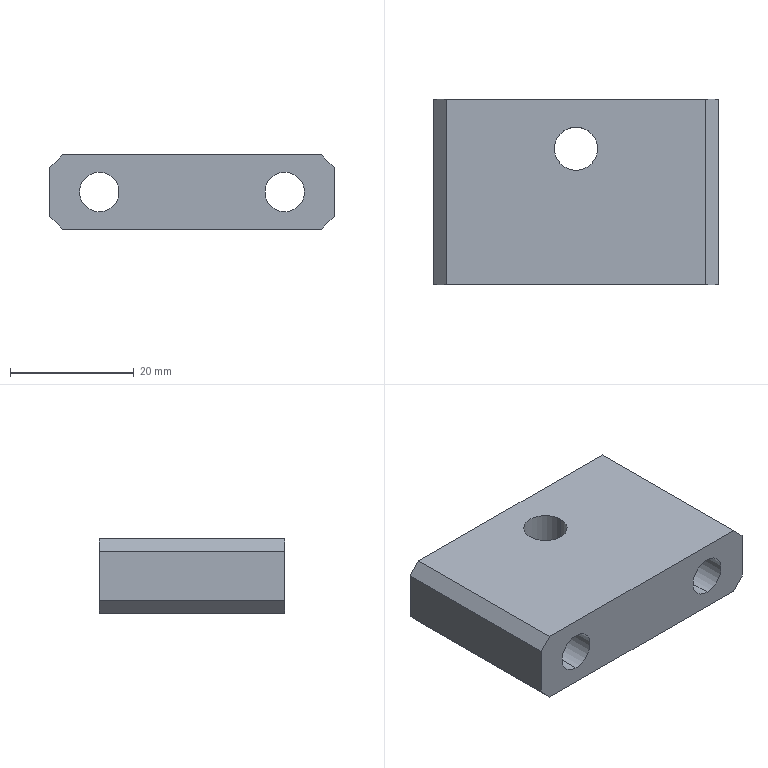Part | SolidWorks | features HoleWzd 2, Chamfer 1, Extrusion 1, ICE 1 | 1 solid | 22 faces | box 46 x 30 x 12 mm | volume 11866 mm3 | plane 12 | cylinder 10 | commonest cylinder face diameters 6.4 x4 11 x4 7 x2
STEP:
#1=CARTESIAN_POINT('',(8.,13.6,0.5));
#2=VERTEX_POINT('',#1);
#3=CARTESIAN_POINT('',(8.,13.6,11.5));
#4=VERTEX_POINT('',#3);
#5=CARTESIAN_POINT('',(8.,13.6,6.));
#6=DIRECTION('',(0.,1.,0.));
#7=DIRECTION('',(0.,0.,1.));
#8=AXIS2_PLACEMENT_3D('',#5,#6,#7);
#9=CIRCLE('',#8,5.5);
#10=EDGE_CURVE('',#2,#4,#9,.T.);
#11=ORIENTED_EDGE('',*,*,#10,.F.);
#12=CARTESIAN_POINT('',(8.,30.,0.5));
#13=VERTEX_POINT('',#12);
#14=CARTESIAN_POINT('',(8.,30.,0.5));
#15=DIRECTION('',(0.,1.,0.));
#16=VECTOR('',#15,1000.);
#17=LINE('',#14,#16);
#18=EDGE_CURVE('',#2,#13,#17,.T.);
#19=ORIENTED_EDGE('',*,*,#18,.T.);
#20=CARTESIAN_POINT('',(8.,30.,11.5));
#21=VERTEX_POINT('',#20);
#22=CARTESIAN_POINT('',(8.,30.,6.));
#23=DIRECTION('',(0.,1.,0.));
#24=DIRECTION('',(0.,0.,1.));
#25=AXIS2_PLACEMENT_3D('',#22,#23,#24);
#26=CIRCLE('',#25,5.5);
#27=EDGE_CURVE('',#13,#21,#26,.T.);
#28=ORIENTED_EDGE('',*,*,#27,.T.);
#29=CARTESIAN_POINT('',(8.,30.,11.5));
#30=DIRECTION('',(0.,1.,0.));
#31=VECTOR('',#30,1000.);
#32=LINE('',#29,#31);
#33=EDGE_CURVE('',#4,#21,#32,.T.);
#34=ORIENTED_EDGE('',*,*,#33,.F.);
#35=EDGE_LOOP('',(#11,#19,#28,#34));
#36=FACE_OUTER_BOUND('',#35,.T.);
#37=CARTESIAN_POINT('',(8.,30.,6.));
#38=DIRECTION('',(0.,1.,0.));
#39=DIRECTION('',(0.,0.,1.));
#40=AXIS2_PLACEMENT_3D('',#37,#38,#39);
#41=CYLINDRICAL_SURFACE('',#40,5.5);
#42=ADVANCED_FACE('',(#36),#41,.F.);
#43=CARTESIAN_POINT('',(38.,13.6,0.5));
#44=VERTEX_POINT('',#43);
#45=CARTESIAN_POINT('',(38.,13.6,11.5));
#46=VERTEX_POINT('',#45);
#47=CARTESIAN_POINT('',(38.,13.6,6.));
#48=DIRECTION('',(0.,1.,0.));
#49=DIRECTION('',(0.,0.,1.));
#50=AXIS2_PLACEMENT_3D('',#47,#48,#49);
#51=CIRCLE('',#50,5.5);
#52=EDGE_CURVE('',#44,#46,#51,.T.);
#53=ORIENTED_EDGE('',*,*,#52,.F.);
#54=CARTESIAN_POINT('',(38.,30.,0.5));
#55=VERTEX_POINT('',#54);
#56=CARTESIAN_POINT('',(38.,30.,0.5));
#57=DIRECTION('',(0.,1.,0.));
#58=VECTOR('',#57,1000.);
#59=LINE('',#56,#58);
#60=EDGE_CURVE('',#44,#55,#59,.T.);
#61=ORIENTED_EDGE('',*,*,#60,.T.);
#62=CARTESIAN_POINT('',(38.,30.,11.5));
#63=VERTEX_POINT('',#62);
#64=CARTESIAN_POINT('',(38.,30.,6.));
#65=DIRECTION('',(0.,1.,0.));
#66=DIRECTION('',(0.,0.,1.));
#67=AXIS2_PLACEMENT_3D('',#64,#65,#66);
#68=CIRCLE('',#67,5.5);
#69=EDGE_CURVE('',#55,#63,#68,.T.);
#70=ORIENTED_EDGE('',*,*,#69,.T.);
#71=CARTESIAN_POINT('',(38.,30.,11.5));
#72=DIRECTION('',(0.,1.,0.));
#73=VECTOR('',#72,1000.);
#74=LINE('',#71,#73);
#75=EDGE_CURVE('',#46,#63,#74,.T.);
#76=ORIENTED_EDGE('',*,*,#75,.F.);
#77=EDGE_LOOP('',(#53,#61,#70,#76));
#78=FACE_OUTER_BOUND('',#77,.T.);
#79=CARTESIAN_POINT('',(38.,30.,6.));
#80=DIRECTION('',(0.,1.,0.));
#81=DIRECTION('',(0.,0.,1.));
#82=AXIS2_PLACEMENT_3D('',#79,#80,#81);
#83=CYLINDRICAL_SURFACE('',#82,5.5);
#84=ADVANCED_FACE('',(#78),#83,.F.);
#85=CARTESIAN_POINT('',(19.5,22.,0.));
#86=VERTEX_POINT('',#85);
#87=CARTESIAN_POINT('',(26.5,22.,0.));
#88=VERTEX_POINT('',#87);
#89=CARTESIAN_POINT('',(23.,22.,0.));
#90=DIRECTION('',(0.,0.,1.));
#91=DIRECTION('',(1.,0.,0.));
#92=AXIS2_PLACEMENT_3D('',#89,#90,#91);
#93=CIRCLE('',#92,3.5);
#94=EDGE_CURVE('',#86,#88,#93,.T.);
#95=ORIENTED_EDGE('',*,*,#94,.F.);
#96=CARTESIAN_POINT('',(19.5,22.,12.));
#97=VERTEX_POINT('',#96);
#98=CARTESIAN_POINT('',(19.5,22.,12.));
#99=DIRECTION('',(0.,0.,1.));
#100=VECTOR('',#99,1000.);
#101=LINE('',#98,#100);
#102=EDGE_CURVE('',#86,#97,#101,.T.);
#103=ORIENTED_EDGE('',*,*,#102,.T.);
#104=CARTESIAN_POINT('',(26.5,22.,12.));
#105=VERTEX_POINT('',#104);
#106=CARTESIAN_POINT('',(23.,22.,12.));
#107=DIRECTION('',(0.,0.,1.));
#108=DIRECTION('',(1.,0.,0.));
#109=AXIS2_PLACEMENT_3D('',#106,#107,#108);
#110=CIRCLE('',#109,3.5);
#111=EDGE_CURVE('',#97,#105,#110,.T.);
#112=ORIENTED_EDGE('',*,*,#111,.T.);
#113=CARTESIAN_POINT('',(26.5,22.,12.));
#114=DIRECTION('',(0.,0.,1.));
#115=VECTOR('',#114,1000.);
#116=LINE('',#113,#115);
#117=EDGE_CURVE('',#88,#105,#116,.T.);
#118=ORIENTED_EDGE('',*,*,#117,.F.);
#119=EDGE_LOOP('',(#95,#103,#112,#118));
#120=FACE_OUTER_BOUND('',#119,.T.);
#121=CARTESIAN_POINT('',(23.,22.,12.));
#122=DIRECTION('',(0.,0.,1.));
#123=DIRECTION('',(1.,0.,0.));
#124=AXIS2_PLACEMENT_3D('',#121,#122,#123);
#125=CYLINDRICAL_SURFACE('',#124,3.5);
#126=ADVANCED_FACE('',(#120),#125,.F.);
#127=CARTESIAN_POINT('',(8.,0.,2.8));
#128=VERTEX_POINT('',#127);
#129=CARTESIAN_POINT('',(8.,0.,9.2));
#130=VERTEX_POINT('',#129);
#131=CARTESIAN_POINT('',(8.,0.,6.));
#132=DIRECTION('',(0.,1.,0.));
#133=DIRECTION('',(0.,0.,1.));
#134=AXIS2_PLACEMENT_3D('',#131,#132,#133);
#135=CIRCLE('',#134,3.2);
#136=EDGE_CURVE('',#128,#130,#135,.T.);
#137=ORIENTED_EDGE('',*,*,#136,.F.);
#138=CARTESIAN_POINT('',(8.,13.6,2.8));
#139=VERTEX_POINT('',#138);
#140=CARTESIAN_POINT('',(8.,30.,2.8));
#141=DIRECTION('',(0.,1.,0.));
#142=VECTOR('',#141,1000.);
#143=LINE('',#140,#142);
#144=EDGE_CURVE('',#128,#139,#143,.T.);
#145=ORIENTED_EDGE('',*,*,#144,.T.);
#146=CARTESIAN_POINT('',(8.,13.6,9.2));
#147=VERTEX_POINT('',#146);
#148=CARTESIAN_POINT('',(8.,13.6,6.));
#149=DIRECTION('',(0.,-1.,0.));
#150=DIRECTION('',(0.,0.,1.));
#151=AXIS2_PLACEMENT_3D('',#148,#149,#150);
#152=CIRCLE('',#151,3.2);
#153=EDGE_CURVE('',#147,#139,#152,.T.);
#154=ORIENTED_EDGE('',*,*,#153,.F.);
#155=CARTESIAN_POINT('',(8.,30.,9.2));
#156=DIRECTION('',(0.,1.,0.));
#157=VECTOR('',#156,1000.);
#158=LINE('',#155,#157);
#159=EDGE_CURVE('',#130,#147,#158,.T.);
#160=ORIENTED_EDGE('',*,*,#159,.F.);
#161=EDGE_LOOP('',(#137,#145,#154,#160));
#162=FACE_OUTER_BOUND('',#161,.T.);
#163=CARTESIAN_POINT('',(8.,30.,6.));
#164=DIRECTION('',(0.,1.,0.));
#165=DIRECTION('',(0.,0.,1.));
#166=AXIS2_PLACEMENT_3D('',#163,#164,#165);
#167=CYLINDRICAL_SURFACE('',#166,3.2);
#168=ADVANCED_FACE('',(#162),#167,.F.);
#169=CARTESIAN_POINT('',(38.,0.,2.8));
#170=VERTEX_POINT('',#169);
#171=CARTESIAN_POINT('',(38.,0.,9.2));
#172=VERTEX_POINT('',#171);
#173=CARTESIAN_POINT('',(38.,0.,6.));
#174=DIRECTION('',(0.,1.,0.));
#175=DIRECTION('',(0.,0.,1.));
#176=AXIS2_PLACEMENT_3D('',#173,#174,#175);
#177=CIRCLE('',#176,3.2);
#178=EDGE_CURVE('',#170,#172,#177,.T.);
#179=ORIENTED_EDGE('',*,*,#178,.F.);
#180=CARTESIAN_POINT('',(38.,13.6,2.8));
#181=VERTEX_POINT('',#180);
#182=CARTESIAN_POINT('',(38.,30.,2.8));
#183=DIRECTION('',(0.,1.,0.));
#184=VECTOR('',#183,1000.);
#185=LINE('',#182,#184);
#186=EDGE_CURVE('',#170,#181,#185,.T.);
#187=ORIENTED_EDGE('',*,*,#186,.T.);
#188=CARTESIAN_POINT('',(38.,13.6,9.2));
#189=VERTEX_POINT('',#188);
#190=CARTESIAN_POINT('',(38.,13.6,6.));
#191=DIRECTION('',(0.,-1.,0.));
#192=DIRECTION('',(0.,0.,1.));
#193=AXIS2_PLACEMENT_3D('',#190,#191,#192);
#194=CIRCLE('',#193,3.2);
#195=EDGE_CURVE('',#189,#181,#194,.T.);
#196=ORIENTED_EDGE('',*,*,#195,.F.);
#197=CARTESIAN_POINT('',(38.,30.,9.2));
#198=DIRECTION('',(0.,1.,0.));
#199=VECTOR('',#198,1000.);
#200=LINE('',#197,#199);
#201=EDGE_CURVE('',#172,#189,#200,.T.);
#202=ORIENTED_EDGE('',*,*,#201,.F.);
#203=EDGE_LOOP('',(#179,#187,#196,#202));
#204=FACE_OUTER_BOUND('',#203,.T.);
#205=CARTESIAN_POINT('',(38.,30.,6.));
#206=DIRECTION('',(0.,1.,0.));
#207=DIRECTION('',(0.,0.,1.));
#208=AXIS2_PLACEMENT_3D('',#205,#206,#207);
#209=CYLINDRICAL_SURFACE('',#208,3.2);
#210=ADVANCED_FACE('',(#204),#209,.F.);
#211=ORIENTED_EDGE('',*,*,#186,.F.);
#212=CARTESIAN_POINT('',(38.,0.,6.));
#213=DIRECTION('',(0.,1.,0.));
#214=DIRECTION('',(0.,0.,1.));
#215=AXIS2_PLACEMENT_3D('',#212,#213,#214);
#216=CIRCLE('',#215,3.2);
#217=EDGE_CURVE('',#172,#170,#216,.T.);
#218=ORIENTED_EDGE('',*,*,#217,.F.);
#219=ORIENTED_EDGE('',*,*,#201,.T.);
#220=CARTESIAN_POINT('',(38.,13.6,6.));
#221=DIRECTION('',(0.,-1.,0.));
#222=DIRECTION('',(0.,0.,1.));
#223=AXIS2_PLACEMENT_3D('',#220,#221,#222);
#224=CIRCLE('',#223,3.2);
#225=EDGE_CURVE('',#181,#189,#224,.T.);
#226=ORIENTED_EDGE('',*,*,#225,.F.);
#227=EDGE_LOOP('',(#211,#218,#219,#226));
#228=FACE_OUTER_BOUND('',#227,.T.);
#229=CARTESIAN_POINT('',(38.,30.,6.));
#230=DIRECTION('',(0.,1.,0.));
#231=DIRECTION('',(0.,0.,1.));
#232=AXIS2_PLACEMENT_3D('',#229,#230,#231);
#233=CYLINDRICAL_SURFACE('',#232,3.2);
#234=ADVANCED_FACE('',(#228),#233,.F.);
#235=ORIENTED_EDGE('',*,*,#144,.F.);
#236=CARTESIAN_POINT('',(8.,0.,6.));
#237=DIRECTION('',(0.,1.,0.));
#238=DIRECTION('',(0.,0.,1.));
#239=AXIS2_PLACEMENT_3D('',#236,#237,#238);
#240=CIRCLE('',#239,3.2);
#241=EDGE_CURVE('',#130,#128,#240,.T.);
#242=ORIENTED_EDGE('',*,*,#241,.F.);
#243=ORIENTED_EDGE('',*,*,#159,.T.);
#244=CARTESIAN_POINT('',(8.,13.6,6.));
#245=DIRECTION('',(0.,-1.,0.));
#246=DIRECTION('',(0.,0.,1.));
#247=AXIS2_PLACEMENT_3D('',#244,#245,#246);
#248=CIRCLE('',#247,3.2);
#249=EDGE_CURVE('',#139,#147,#248,.T.);
#250=ORIENTED_EDGE('',*,*,#249,.F.);
#251=EDGE_LOOP('',(#235,#242,#243,#250));
#252=FACE_OUTER_BOUND('',#251,.T.);
#253=CARTESIAN_POINT('',(8.,30.,6.));
#254=DIRECTION('',(0.,1.,0.));
#255=DIRECTION('',(0.,0.,1.));
#256=AXIS2_PLACEMENT_3D('',#253,#254,#255);
#257=CYLINDRICAL_SURFACE('',#256,3.2);
#258=ADVANCED_FACE('',(#252),#257,.F.);
#259=CARTESIAN_POINT('',(0.,0.,10.));
#260=VERTEX_POINT('',#259);
#261=CARTESIAN_POINT('',(0.,0.,2.));
#262=VERTEX_POINT('',#261);
#263=CARTESIAN_POINT('',(0.,0.,12.));
#264=DIRECTION('',(0.,0.,-1.));
#265=VECTOR('',#264,1000.);
#266=LINE('',#263,#265);
#267=EDGE_CURVE('',#260,#262,#266,.T.);
#268=ORIENTED_EDGE('',*,*,#267,.F.);
#269=CARTESIAN_POINT('',(0.,30.,10.));
#270=VERTEX_POINT('',#269);
#271=CARTESIAN_POINT('',(0.,0.,10.));
#272=DIRECTION('',(0.,1.,0.));
#273=VECTOR('',#272,1000.);
#274=LINE('',#271,#273);
#275=EDGE_CURVE('',#260,#270,#274,.T.);
#276=ORIENTED_EDGE('',*,*,#275,.T.);
#277=CARTESIAN_POINT('',(0.,30.,2.));
#278=VERTEX_POINT('',#277);
#279=CARTESIAN_POINT('',(0.,30.,12.));
#280=DIRECTION('',(0.,0.,-1.));
#281=VECTOR('',#280,1000.);
#282=LINE('',#279,#281);
#283=EDGE_CURVE('',#270,#278,#282,.T.);
#284=ORIENTED_EDGE('',*,*,#283,.T.);
#285=CARTESIAN_POINT('',(0.,0.,2.));
#286=DIRECTION('',(0.,-1.,0.));
#287=VECTOR('',#286,1000.);
#288=LINE('',#285,#287);
#289=EDGE_CURVE('',#278,#262,#288,.T.);
#290=ORIENTED_EDGE('',*,*,#289,.T.);
#291=EDGE_LOOP('',(#268,#276,#284,#290));
#292=FACE_OUTER_BOUND('',#291,.T.);
#293=CARTESIAN_POINT('',(0.,0.,12.));
#294=DIRECTION('',(1.,0.,0.));
#295=DIRECTION('',(0.,0.,-1.));
#296=AXIS2_PLACEMENT_3D('',#293,#294,#295);
#297=PLANE('',#296);
#298=ADVANCED_FACE('',(#292),#297,.F.);
#299=ORIENTED_EDGE('',*,*,#241,.T.);
#300=ORIENTED_EDGE('',*,*,#136,.T.);
#301=EDGE_LOOP('',(#299,#300));
#302=FACE_BOUND('',#301,.T.);
#303=ORIENTED_EDGE('',*,*,#217,.T.);
#304=ORIENTED_EDGE('',*,*,#178,.T.);
#305=EDGE_LOOP('',(#303,#304));
#306=FACE_BOUND('',#305,.T.);
#307=CARTESIAN_POINT('',(2.,0.,12.));
#308=VERTEX_POINT('',#307);
#309=CARTESIAN_POINT('',(44.,0.,12.));
#310=VERTEX_POINT('',#309);
#311=CARTESIAN_POINT('',(0.,0.,12.));
#312=DIRECTION('',(1.,0.,0.));
#313=VECTOR('',#312,1000.);
#314=LINE('',#311,#313);
#315=EDGE_CURVE('',#308,#310,#314,.T.);
#316=ORIENTED_EDGE('',*,*,#315,.F.);
#317=CARTESIAN_POINT('',(2.,0.,12.));
#318=DIRECTION('',(-0.7071,0.,-0.7071));
#319=VECTOR('',#318,1000.);
#320=LINE('',#317,#319);
#321=EDGE_CURVE('',#308,#260,#320,.T.);
#322=ORIENTED_EDGE('',*,*,#321,.T.);
#323=ORIENTED_EDGE('',*,*,#267,.T.);
#324=CARTESIAN_POINT('',(2.,0.,0.));
#325=VERTEX_POINT('',#324);
#326=CARTESIAN_POINT('',(0.,0.,2.));
#327=DIRECTION('',(0.7071,0.,-0.7071));
#328=VECTOR('',#327,1000.);
#329=LINE('',#326,#328);
#330=EDGE_CURVE('',#262,#325,#329,.T.);
#331=ORIENTED_EDGE('',*,*,#330,.T.);
#332=CARTESIAN_POINT('',(44.,0.,0.));
#333=VERTEX_POINT('',#332);
#334=CARTESIAN_POINT('',(0.,0.,0.));
#335=DIRECTION('',(1.,0.,0.));
#336=VECTOR('',#335,1000.);
#337=LINE('',#334,#336);
#338=EDGE_CURVE('',#325,#333,#337,.T.);
#339=ORIENTED_EDGE('',*,*,#338,.T.);
#340=CARTESIAN_POINT('',(46.,0.,2.));
#341=VERTEX_POINT('',#340);
#342=CARTESIAN_POINT('',(46.,0.,2.));
#343=DIRECTION('',(0.7071,0.,0.7071));
#344=VECTOR('',#343,1000.);
#345=LINE('',#342,#344);
#346=EDGE_CURVE('',#333,#341,#345,.T.);
#347=ORIENTED_EDGE('',*,*,#346,.T.);
#348=CARTESIAN_POINT('',(46.,0.,10.));
#349=VERTEX_POINT('',#348);
#350=CARTESIAN_POINT('',(46.,0.,12.));
#351=DIRECTION('',(0.,0.,-1.));
#352=VECTOR('',#351,1000.);
#353=LINE('',#350,#352);
#354=EDGE_CURVE('',#349,#341,#353,.T.);
#355=ORIENTED_EDGE('',*,*,#354,.F.);
#356=CARTESIAN_POINT('',(44.,0.,12.));
#357=DIRECTION('',(-0.7071,0.,0.7071));
#358=VECTOR('',#357,1000.);
#359=LINE('',#356,#358);
#360=EDGE_CURVE('',#349,#310,#359,.T.);
#361=ORIENTED_EDGE('',*,*,#360,.T.);
#362=EDGE_LOOP('',(#316,#322,#323,#331,#339,#347,#355,#361));
#363=FACE_OUTER_BOUND('',#362,.T.);
#364=CARTESIAN_POINT('',(0.,0.,12.));
#365=DIRECTION('',(0.,1.,0.));
#366=DIRECTION('',(0.,0.,1.));
#367=AXIS2_PLACEMENT_3D('',#364,#365,#366);
#368=PLANE('',#367);
#369=ADVANCED_FACE('',(#302,#306,#363),#368,.F.);
#370=CARTESIAN_POINT('',(46.,30.,10.));
#371=VERTEX_POINT('',#370);
#372=CARTESIAN_POINT('',(46.,30.,2.));
#373=VERTEX_POINT('',#372);
#374=CARTESIAN_POINT('',(46.,30.,12.));
#375=DIRECTION('',(0.,0.,-1.));
#376=VECTOR('',#375,1000.);
#377=LINE('',#374,#376);
#378=EDGE_CURVE('',#371,#373,#377,.T.);
#379=ORIENTED_EDGE('',*,*,#378,.F.);
#380=CARTESIAN_POINT('',(46.,0.,10.));
#381=DIRECTION('',(0.,-1.,0.));
#382=VECTOR('',#381,1000.);
#383=LINE('',#380,#382);
#384=EDGE_CURVE('',#371,#349,#383,.T.);
#385=ORIENTED_EDGE('',*,*,#384,.T.);
#386=ORIENTED_EDGE('',*,*,#354,.T.);
#387=CARTESIAN_POINT('',(46.,30.,2.));
#388=DIRECTION('',(0.,1.,0.));
#389=VECTOR('',#388,1000.);
#390=LINE('',#387,#389);
#391=EDGE_CURVE('',#341,#373,#390,.T.);
#392=ORIENTED_EDGE('',*,*,#391,.T.);
#393=EDGE_LOOP('',(#379,#385,#386,#392));
#394=FACE_OUTER_BOUND('',#393,.T.);
#395=CARTESIAN_POINT('',(46.,0.,12.));
#396=DIRECTION('',(-1.,0.,0.));
#397=DIRECTION('',(0.,0.,1.));
#398=AXIS2_PLACEMENT_3D('',#395,#396,#397);
#399=PLANE('',#398);
#400=ADVANCED_FACE('',(#394),#399,.F.);
#401=CARTESIAN_POINT('',(8.,30.,6.));
#402=DIRECTION('',(0.,1.,0.));
#403=DIRECTION('',(0.,0.,1.));
#404=AXIS2_PLACEMENT_3D('',#401,#402,#403);
#405=CIRCLE('',#404,5.5);
#406=EDGE_CURVE('',#21,#13,#405,.T.);
#407=ORIENTED_EDGE('',*,*,#406,.F.);
#408=ORIENTED_EDGE('',*,*,#27,.F.);
#409=EDGE_LOOP('',(#407,#408));
#410=FACE_BOUND('',#409,.T.);
#411=CARTESIAN_POINT('',(38.,30.,6.));
#412=DIRECTION('',(0.,1.,0.));
#413=DIRECTION('',(0.,0.,1.));
#414=AXIS2_PLACEMENT_3D('',#411,#412,#413);
#415=CIRCLE('',#414,5.5);
#416=EDGE_CURVE('',#63,#55,#415,.T.);
#417=ORIENTED_EDGE('',*,*,#416,.F.);
#418=ORIENTED_EDGE('',*,*,#69,.F.);
#419=EDGE_LOOP('',(#417,#418));
#420=FACE_BOUND('',#419,.T.);
#421=ORIENTED_EDGE('',*,*,#283,.F.);
#422=CARTESIAN_POINT('',(2.,30.,12.));
#423=VERTEX_POINT('',#422);
#424=CARTESIAN_POINT('',(2.,30.,12.));
#425=DIRECTION('',(0.7071,0.,0.7071));
#426=VECTOR('',#425,1000.);
#427=LINE('',#424,#426);
#428=EDGE_CURVE('',#270,#423,#427,.T.);
#429=ORIENTED_EDGE('',*,*,#428,.T.);
#430=CARTESIAN_POINT('',(44.,30.,12.));
#431=VERTEX_POINT('',#430);
#432=CARTESIAN_POINT('',(0.,30.,12.));
#433=DIRECTION('',(-1.,0.,0.));
#434=VECTOR('',#433,1000.);
#435=LINE('',#432,#434);
#436=EDGE_CURVE('',#431,#423,#435,.T.);
#437=ORIENTED_EDGE('',*,*,#436,.F.);
#438=CARTESIAN_POINT('',(44.,30.,12.));
#439=DIRECTION('',(0.7071,0.,-0.7071));
#440=VECTOR('',#439,1000.);
#441=LINE('',#438,#440);
#442=EDGE_CURVE('',#431,#371,#441,.T.);
#443=ORIENTED_EDGE('',*,*,#442,.T.);
#444=ORIENTED_EDGE('',*,*,#378,.T.);
#445=CARTESIAN_POINT('',(44.,30.,0.));
#446=VERTEX_POINT('',#445);
#447=CARTESIAN_POINT('',(46.,30.,2.));
#448=DIRECTION('',(-0.7071,0.,-0.7071));
#449=VECTOR('',#448,1000.);
#450=LINE('',#447,#449);
#451=EDGE_CURVE('',#373,#446,#450,.T.);
#452=ORIENTED_EDGE('',*,*,#451,.T.);
#453=CARTESIAN_POINT('',(2.,30.,0.));
#454=VERTEX_POINT('',#453);
#455=CARTESIAN_POINT('',(0.,30.,0.));
#456=DIRECTION('',(-1.,0.,0.));
#457=VECTOR('',#456,1000.);
#458=LINE('',#455,#457);
#459=EDGE_CURVE('',#446,#454,#458,.T.);
#460=ORIENTED_EDGE('',*,*,#459,.T.);
#461=CARTESIAN_POINT('',(0.,30.,2.));
#462=DIRECTION('',(-0.7071,0.,0.7071));
#463=VECTOR('',#462,1000.);
#464=LINE('',#461,#463);
#465=EDGE_CURVE('',#454,#278,#464,.T.);
#466=ORIENTED_EDGE('',*,*,#465,.T.);
#467=EDGE_LOOP('',(#421,#429,#437,#443,#444,#452,#460,#466));
#468=FACE_OUTER_BOUND('',#467,.T.);
#469=CARTESIAN_POINT('',(0.,30.,12.));
#470=DIRECTION('',(0.,-1.,0.));
#471=DIRECTION('',(0.,0.,-1.));
#472=AXIS2_PLACEMENT_3D('',#469,#470,#471);
#473=PLANE('',#472);
#474=ADVANCED_FACE('',(#410,#420,#468),#473,.F.);
#475=CARTESIAN_POINT('',(23.,22.,12.));
#476=DIRECTION('',(0.,0.,1.));
#477=DIRECTION('',(1.,0.,0.));
#478=AXIS2_PLACEMENT_3D('',#475,#476,#477);
#479=CIRCLE('',#478,3.5);
#480=EDGE_CURVE('',#105,#97,#479,.T.);
#481=ORIENTED_EDGE('',*,*,#480,.F.);
#482=ORIENTED_EDGE('',*,*,#111,.F.);
#483=EDGE_LOOP('',(#481,#482));
#484=FACE_BOUND('',#483,.T.);
#485=ORIENTED_EDGE('',*,*,#436,.T.);
#486=CARTESIAN_POINT('',(2.,0.,12.));
#487=DIRECTION('',(0.,-1.,0.));
#488=VECTOR('',#487,1000.);
#489=LINE('',#486,#488);
#490=EDGE_CURVE('',#423,#308,#489,.T.);
#491=ORIENTED_EDGE('',*,*,#490,.T.);
#492=ORIENTED_EDGE('',*,*,#315,.T.);
#493=CARTESIAN_POINT('',(44.,0.,12.));
#494=DIRECTION('',(0.,1.,0.));
#495=VECTOR('',#494,1000.);
#496=LINE('',#493,#495);
#497=EDGE_CURVE('',#310,#431,#496,.T.);
#498=ORIENTED_EDGE('',*,*,#497,.T.);
#499=EDGE_LOOP('',(#485,#491,#492,#498));
#500=FACE_OUTER_BOUND('',#499,.T.);
#501=CARTESIAN_POINT('',(0.,0.,12.));
#502=DIRECTION('',(0.,0.,-1.));
#503=DIRECTION('',(-1.,0.,0.));
#504=AXIS2_PLACEMENT_3D('',#501,#502,#503);
#505=PLANE('',#504);
#506=ADVANCED_FACE('',(#484,#500),#505,.F.);
#507=CARTESIAN_POINT('',(23.,22.,0.));
#508=DIRECTION('',(0.,0.,1.));
#509=DIRECTION('',(1.,0.,0.));
#510=AXIS2_PLACEMENT_3D('',#507,#508,#509);
#511=CIRCLE('',#510,3.5);
#512=EDGE_CURVE('',#88,#86,#511,.T.);
#513=ORIENTED_EDGE('',*,*,#512,.T.);
#514=ORIENTED_EDGE('',*,*,#94,.T.);
#515=EDGE_LOOP('',(#513,#514));
#516=FACE_BOUND('',#515,.T.);
#517=ORIENTED_EDGE('',*,*,#338,.F.);
#518=CARTESIAN_POINT('',(2.,30.,0.));
#519=DIRECTION('',(0.,1.,0.));
#520=VECTOR('',#519,1000.);
#521=LINE('',#518,#520);
#522=EDGE_CURVE('',#325,#454,#521,.T.);
#523=ORIENTED_EDGE('',*,*,#522,.T.);
#524=ORIENTED_EDGE('',*,*,#459,.F.);
#525=CARTESIAN_POINT('',(44.,0.,0.));
#526=DIRECTION('',(0.,-1.,0.));
#527=VECTOR('',#526,1000.);
#528=LINE('',#525,#527);
#529=EDGE_CURVE('',#446,#333,#528,.T.);
#530=ORIENTED_EDGE('',*,*,#529,.T.);
#531=EDGE_LOOP('',(#517,#523,#524,#530));
#532=FACE_OUTER_BOUND('',#531,.T.);
#533=CARTESIAN_POINT('',(0.,0.,0.));
#534=DIRECTION('',(0.,0.,-1.));
#535=DIRECTION('',(-1.,0.,0.));
#536=AXIS2_PLACEMENT_3D('',#533,#534,#535);
#537=PLANE('',#536);
#538=ADVANCED_FACE('',(#516,#532),#537,.T.);
#539=ORIENTED_EDGE('',*,*,#102,.F.);
#540=ORIENTED_EDGE('',*,*,#512,.F.);
#541=ORIENTED_EDGE('',*,*,#117,.T.);
#542=ORIENTED_EDGE('',*,*,#480,.T.);
#543=EDGE_LOOP('',(#539,#540,#541,#542));
#544=FACE_OUTER_BOUND('',#543,.T.);
#545=CARTESIAN_POINT('',(23.,22.,12.));
#546=DIRECTION('',(0.,0.,1.));
#547=DIRECTION('',(1.,0.,0.));
#548=AXIS2_PLACEMENT_3D('',#545,#546,#547);
#549=CYLINDRICAL_SURFACE('',#548,3.5);
#550=ADVANCED_FACE('',(#544),#549,.F.);
#551=ORIENTED_EDGE('',*,*,#60,.F.);
#552=CARTESIAN_POINT('',(38.,13.6,6.));
#553=DIRECTION('',(0.,1.,0.));
#554=DIRECTION('',(0.,0.,1.));
#555=AXIS2_PLACEMENT_3D('',#552,#553,#554);
#556=CIRCLE('',#555,5.5);
#557=EDGE_CURVE('',#46,#44,#556,.T.);
#558=ORIENTED_EDGE('',*,*,#557,.F.);
#559=ORIENTED_EDGE('',*,*,#75,.T.);
#560=ORIENTED_EDGE('',*,*,#416,.T.);
#561=EDGE_LOOP('',(#551,#558,#559,#560));
#562=FACE_OUTER_BOUND('',#561,.T.);
#563=CARTESIAN_POINT('',(38.,30.,6.));
#564=DIRECTION('',(0.,1.,0.));
#565=DIRECTION('',(0.,0.,1.));
#566=AXIS2_PLACEMENT_3D('',#563,#564,#565);
#567=CYLINDRICAL_SURFACE('',#566,5.5);
#568=ADVANCED_FACE('',(#562),#567,.F.);
#569=ORIENTED_EDGE('',*,*,#18,.F.);
#570=CARTESIAN_POINT('',(8.,13.6,6.));
#571=DIRECTION('',(0.,1.,0.));
#572=DIRECTION('',(0.,0.,1.));
#573=AXIS2_PLACEMENT_3D('',#570,#571,#572);
#574=CIRCLE('',#573,5.5);
#575=EDGE_CURVE('',#4,#2,#574,.T.);
#576=ORIENTED_EDGE('',*,*,#575,.F.);
#577=ORIENTED_EDGE('',*,*,#33,.T.);
#578=ORIENTED_EDGE('',*,*,#406,.T.);
#579=EDGE_LOOP('',(#569,#576,#577,#578));
#580=FACE_OUTER_BOUND('',#579,.T.);
#581=CARTESIAN_POINT('',(8.,30.,6.));
#582=DIRECTION('',(0.,1.,0.));
#583=DIRECTION('',(0.,0.,1.));
#584=AXIS2_PLACEMENT_3D('',#581,#582,#583);
#585=CYLINDRICAL_SURFACE('',#584,5.5);
#586=ADVANCED_FACE('',(#580),#585,.F.);
#587=ORIENTED_EDGE('',*,*,#575,.T.);
#588=ORIENTED_EDGE('',*,*,#10,.T.);
#589=EDGE_LOOP('',(#587,#588));
#590=FACE_OUTER_BOUND('',#589,.T.);
#591=ORIENTED_EDGE('',*,*,#153,.T.);
#592=ORIENTED_EDGE('',*,*,#249,.T.);
#593=EDGE_LOOP('',(#591,#592));
#594=FACE_BOUND('',#593,.T.);
#595=CARTESIAN_POINT('',(8.,13.6,6.));
#596=DIRECTION('',(0.,1.,0.));
#597=DIRECTION('',(0.,0.,1.));
#598=AXIS2_PLACEMENT_3D('',#595,#596,#597);
#599=PLANE('',#598);
#600=ADVANCED_FACE('',(#590,#594),#599,.T.);
#601=ORIENTED_EDGE('',*,*,#557,.T.);
#602=ORIENTED_EDGE('',*,*,#52,.T.);
#603=EDGE_LOOP('',(#601,#602));
#604=FACE_OUTER_BOUND('',#603,.T.);
#605=ORIENTED_EDGE('',*,*,#195,.T.);
#606=ORIENTED_EDGE('',*,*,#225,.T.);
#607=EDGE_LOOP('',(#605,#606));
#608=FACE_BOUND('',#607,.T.);
#609=CARTESIAN_POINT('',(38.,13.6,6.));
#610=DIRECTION('',(0.,1.,0.));
#611=DIRECTION('',(0.,0.,1.));
#612=AXIS2_PLACEMENT_3D('',#609,#610,#611);
#613=PLANE('',#612);
#614=ADVANCED_FACE('',(#604,#608),#613,.T.);
#615=ORIENTED_EDGE('',*,*,#428,.F.);
#616=ORIENTED_EDGE('',*,*,#275,.F.);
#617=ORIENTED_EDGE('',*,*,#321,.F.);
#618=ORIENTED_EDGE('',*,*,#490,.F.);
#619=EDGE_LOOP('',(#615,#616,#617,#618));
#620=FACE_OUTER_BOUND('',#619,.T.);
#621=CARTESIAN_POINT('',(2.,0.,12.));
#622=DIRECTION('',(0.7071,0.,-0.7071));
#623=DIRECTION('',(0.,-1.,0.));
#624=AXIS2_PLACEMENT_3D('',#621,#622,#623);
#625=PLANE('',#624);
#626=ADVANCED_FACE('',(#620),#625,.F.);
#627=ORIENTED_EDGE('',*,*,#465,.F.);
#628=ORIENTED_EDGE('',*,*,#522,.F.);
#629=ORIENTED_EDGE('',*,*,#330,.F.);
#630=ORIENTED_EDGE('',*,*,#289,.F.);
#631=EDGE_LOOP('',(#627,#628,#629,#630));
#632=FACE_OUTER_BOUND('',#631,.T.);
#633=CARTESIAN_POINT('',(0.,0.,2.));
#634=DIRECTION('',(-0.7071,0.,-0.7071));
#635=DIRECTION('',(0.,1.,0.));
#636=AXIS2_PLACEMENT_3D('',#633,#634,#635);
#637=PLANE('',#636);
#638=ADVANCED_FACE('',(#632),#637,.T.);
#639=ORIENTED_EDGE('',*,*,#360,.F.);
#640=ORIENTED_EDGE('',*,*,#384,.F.);
#641=ORIENTED_EDGE('',*,*,#442,.F.);
#642=ORIENTED_EDGE('',*,*,#497,.F.);
#643=EDGE_LOOP('',(#639,#640,#641,#642));
#644=FACE_OUTER_BOUND('',#643,.T.);
#645=CARTESIAN_POINT('',(44.,0.,12.));
#646=DIRECTION('',(-0.7071,0.,-0.7071));
#647=DIRECTION('',(0.,1.,0.));
#648=AXIS2_PLACEMENT_3D('',#645,#646,#647);
#649=PLANE('',#648);
#650=ADVANCED_FACE('',(#644),#649,.F.);
#651=ORIENTED_EDGE('',*,*,#346,.F.);
#652=ORIENTED_EDGE('',*,*,#529,.F.);
#653=ORIENTED_EDGE('',*,*,#451,.F.);
#654=ORIENTED_EDGE('',*,*,#391,.F.);
#655=EDGE_LOOP('',(#651,#652,#653,#654));
#656=FACE_OUTER_BOUND('',#655,.T.);
#657=CARTESIAN_POINT('',(46.,0.,2.));
#658=DIRECTION('',(0.7071,0.,-0.7071));
#659=DIRECTION('',(0.,-1.,0.));
#660=AXIS2_PLACEMENT_3D('',#657,#658,#659);
#661=PLANE('',#660);
#662=ADVANCED_FACE('',(#656),#661,.T.);
#663=CLOSED_SHELL('',(#42,#84,#126,#168,#210,#234,#258,#298,#369,#400,#474,#506,#538,#550,#568,#586,#600,#614,#626,#638,#650,#662));
#664=MANIFOLD_SOLID_BREP('',#663);
#665=CARTESIAN_POINT('',(0.,0.,0.));
#666=DIRECTION('',(0.,0.,1.));
#667=DIRECTION('',(1.,0.,0.));
#668=AXIS2_PLACEMENT_3D('',#665,#666,#667);
#669=(LENGTH_UNIT()NAMED_UNIT(*)SI_UNIT(.MILLI.,.METRE.));
#670=UNCERTAINTY_MEASURE_WITH_UNIT(LENGTH_MEASURE(0.00001),#669,'','');
#671=(NAMED_UNIT(*)PLANE_ANGLE_UNIT()SI_UNIT($,.RADIAN.));
#672=(NAMED_UNIT(*)SI_UNIT($,.STERADIAN.)SOLID_ANGLE_UNIT());
#673=(GEOMETRIC_REPRESENTATION_CONTEXT(3)GLOBAL_UNCERTAINTY_ASSIGNED_CONTEXT((#670))GLOBAL_UNIT_ASSIGNED_CONTEXT((#669,#671,#672))REPRESENTATION_CONTEXT('',''));
#674=ADVANCED_BREP_SHAPE_REPRESENTATION('',(#664,#668),#673);